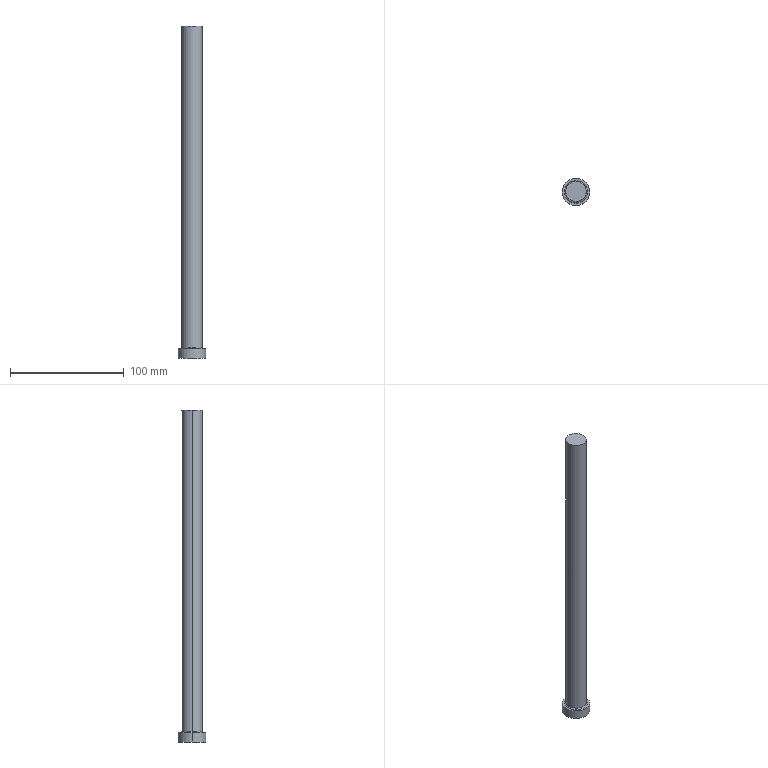Part | STEP file | Pino extrator A - A_18x315 | 1 solid | 9 faces | box 24 x 24 x 292 mm | volume 75901 mm3 | cylinder 4 | plane 3 | torus 2 | commonest cylinder face diameters 18 x2 24 x2
STEP:
#1=CARTESIAN_POINT('',(0.,0.,0.));
#2=DIRECTION('',(0.,0.,1.));
#3=DIRECTION('',(1.,0.,0.));
#4=AXIS2_PLACEMENT_3D('',#1,#2,#3);
#5=CARTESIAN_POINT('',(9.,0.,9.));
#6=VERTEX_POINT('',#5);
#7=CARTESIAN_POINT('',(10.,0.,8.));
#8=VERTEX_POINT('',#7);
#9=CARTESIAN_POINT('',(10.,0.,9.));
#10=DIRECTION('',(0.,-1.,0.));
#11=DIRECTION('',(0.,0.,-1.));
#12=AXIS2_PLACEMENT_3D('',#9,#10,#11);
#13=CIRCLE('',#12,1.);
#14=CARTESIAN_POINT('',(0.,0.,9.));
#15=DIRECTION('',(0.,0.,1.));
#16=DIRECTION('',(1.,0.,0.));
#17=AXIS2_PLACEMENT_3D('',#14,#15,#16);
#18=TOROIDAL_SURFACE('',#17,10.,1.);
#19=CARTESIAN_POINT('',(6.283,-1.571));
#20=DIRECTION('',(0.,1.));
#21=VECTOR('',#20,1.);
#22=LINE('',#19,#21);
#23=(GEOMETRIC_REPRESENTATION_CONTEXT(2)PARAMETRIC_REPRESENTATION_CONTEXT()REPRESENTATION_CONTEXT('',''));
#24=DEFINITIONAL_REPRESENTATION('',(#22),#23);
#25=PCURVE('',#18,#24);
#26=CARTESIAN_POINT('',(0.,0.,9.));
#27=DIRECTION('',(0.,0.,1.));
#28=DIRECTION('',(1.,0.,0.));
#29=AXIS2_PLACEMENT_3D('',#26,#27,#28);
#30=TOROIDAL_SURFACE('',#29,10.,1.);
#31=CARTESIAN_POINT('',(0.,-1.571));
#32=DIRECTION('',(0.,1.));
#33=VECTOR('',#32,1.);
#34=LINE('',#31,#33);
#35=(GEOMETRIC_REPRESENTATION_CONTEXT(2)PARAMETRIC_REPRESENTATION_CONTEXT()REPRESENTATION_CONTEXT('',''));
#36=DEFINITIONAL_REPRESENTATION('',(#34),#35);
#37=PCURVE('',#30,#36);
#38=SURFACE_CURVE('',#13,(#25,#37),.PCURVE_S1.);
#39=EDGE_CURVE('',#6,#8,#38,.T.);
#40=ORIENTED_EDGE('',*,*,#39,.T.);
#41=CARTESIAN_POINT('',(-10.,0.,8.));
#42=VERTEX_POINT('',#41);
#43=CARTESIAN_POINT('',(0.,0.,8.));
#44=DIRECTION('',(0.,0.,-1.));
#45=DIRECTION('',(1.,0.,0.));
#46=AXIS2_PLACEMENT_3D('',#43,#44,#45);
#47=CIRCLE('',#46,10.);
#48=CARTESIAN_POINT('',(6.283,4.712));
#49=DIRECTION('',(-1.,0.));
#50=VECTOR('',#49,1.);
#51=LINE('',#48,#50);
#52=(GEOMETRIC_REPRESENTATION_CONTEXT(2)PARAMETRIC_REPRESENTATION_CONTEXT()REPRESENTATION_CONTEXT('',''));
#53=DEFINITIONAL_REPRESENTATION('',(#51),#52);
#54=PCURVE('',#18,#53);
#55=CARTESIAN_POINT('',(12.,0.,8.));
#56=DIRECTION('',(0.,0.,1.));
#57=DIRECTION('',(1.,0.,0.));
#58=AXIS2_PLACEMENT_3D('',#55,#56,#57);
#59=PLANE('',#58);
#60=CARTESIAN_POINT('',(-2.,0.));
#61=CARTESIAN_POINT('',(-2.,-17.321));
#62=CARTESIAN_POINT('',(-17.,-8.66));
#63=CARTESIAN_POINT('',(-32.,0.));
#64=CARTESIAN_POINT('',(-17.,8.66));
#65=CARTESIAN_POINT('',(-2.,17.321));
#66=CARTESIAN_POINT('',(-2.,0.));
#67=(BOUNDED_CURVE()B_SPLINE_CURVE(2,(#60,#61,#62,#63,#64,#65,#66),.UNSPECIFIED.,.T.,.F.)B_SPLINE_CURVE_WITH_KNOTS((1,2,2,2,2,1),(-2.094,0.,2.094,4.189,6.283,8.378),.UNSPECIFIED.)CURVE()GEOMETRIC_REPRESENTATION_ITEM()RATIONAL_B_SPLINE_CURVE((1.,0.5,1.,0.5,1.,0.5,1.))REPRESENTATION_ITEM(''));
#68=(GEOMETRIC_REPRESENTATION_CONTEXT(2)PARAMETRIC_REPRESENTATION_CONTEXT()REPRESENTATION_CONTEXT('',''));
#69=DEFINITIONAL_REPRESENTATION('',(#67),#68);
#70=PCURVE('',#59,#69);
#71=SURFACE_CURVE('',#47,(#54,#70),.PCURVE_S1.);
#72=EDGE_CURVE('',#8,#42,#71,.T.);
#73=ORIENTED_EDGE('',*,*,#72,.T.);
#74=CARTESIAN_POINT('',(-9.,0.,9.));
#75=VERTEX_POINT('',#74);
#76=CARTESIAN_POINT('',(-10.,0.,9.));
#77=DIRECTION('',(0.,1.,0.));
#78=DIRECTION('',(-1.,0.,0.));
#79=AXIS2_PLACEMENT_3D('',#76,#77,#78);
#80=CIRCLE('',#79,1.);
#81=CARTESIAN_POINT('',(3.142,0.));
#82=DIRECTION('',(0.,1.));
#83=VECTOR('',#82,1.);
#84=LINE('',#81,#83);
#85=(GEOMETRIC_REPRESENTATION_CONTEXT(2)PARAMETRIC_REPRESENTATION_CONTEXT()REPRESENTATION_CONTEXT('',''));
#86=DEFINITIONAL_REPRESENTATION('',(#84),#85);
#87=PCURVE('',#18,#86);
#88=CARTESIAN_POINT('',(3.142,0.));
#89=DIRECTION('',(0.,1.));
#90=VECTOR('',#89,1.);
#91=LINE('',#88,#90);
#92=(GEOMETRIC_REPRESENTATION_CONTEXT(2)PARAMETRIC_REPRESENTATION_CONTEXT()REPRESENTATION_CONTEXT('',''));
#93=DEFINITIONAL_REPRESENTATION('',(#91),#92);
#94=PCURVE('',#30,#93);
#95=SURFACE_CURVE('',#80,(#87,#94),.PCURVE_S1.);
#96=EDGE_CURVE('',#75,#42,#95,.T.);
#97=ORIENTED_EDGE('',*,*,#96,.F.);
#98=CARTESIAN_POINT('',(0.,0.,9.));
#99=DIRECTION('',(0.,0.,1.));
#100=DIRECTION('',(1.,0.,0.));
#101=AXIS2_PLACEMENT_3D('',#98,#99,#100);
#102=CIRCLE('',#101,9.);
#103=CARTESIAN_POINT('',(0.,3.142));
#104=DIRECTION('',(1.,0.));
#105=VECTOR('',#104,1.);
#106=LINE('',#103,#105);
#107=(GEOMETRIC_REPRESENTATION_CONTEXT(2)PARAMETRIC_REPRESENTATION_CONTEXT()REPRESENTATION_CONTEXT('',''));
#108=DEFINITIONAL_REPRESENTATION('',(#106),#107);
#109=PCURVE('',#18,#108);
#110=CARTESIAN_POINT('',(0.,0.,0.));
#111=DIRECTION('',(0.,0.,-1.));
#112=DIRECTION('',(-1.,0.,0.));
#113=AXIS2_PLACEMENT_3D('',#110,#111,#112);
#114=CYLINDRICAL_SURFACE('',#113,9.);
#115=CARTESIAN_POINT('',(9.425,-9.));
#116=DIRECTION('',(-1.,0.));
#117=VECTOR('',#116,1.);
#118=LINE('',#115,#117);
#119=(GEOMETRIC_REPRESENTATION_CONTEXT(2)PARAMETRIC_REPRESENTATION_CONTEXT()REPRESENTATION_CONTEXT('',''));
#120=DEFINITIONAL_REPRESENTATION('',(#118),#119);
#121=PCURVE('',#114,#120);
#122=SURFACE_CURVE('',#102,(#109,#121),.PCURVE_S1.);
#123=EDGE_CURVE('',#75,#6,#122,.T.);
#124=ORIENTED_EDGE('',*,*,#123,.T.);
#125=EDGE_LOOP('',(#40,#73,#97,#124));
#126=FACE_BOUND('',#125,.F.);
#127=ADVANCED_FACE('',(#126),#18,.F.);
#128=CARTESIAN_POINT('',(-12.,0.,8.));
#129=VERTEX_POINT('',#128);
#130=CARTESIAN_POINT('',(12.,0.,8.));
#131=VERTEX_POINT('',#130);
#132=CARTESIAN_POINT('',(0.,0.,8.));
#133=DIRECTION('',(0.,0.,-1.));
#134=DIRECTION('',(-1.,0.,0.));
#135=AXIS2_PLACEMENT_3D('',#132,#133,#134);
#136=CIRCLE('',#135,12.);
#137=CARTESIAN_POINT('',(0.,0.,0.));
#138=DIRECTION('',(0.,0.,-1.));
#139=DIRECTION('',(-1.,0.,0.));
#140=AXIS2_PLACEMENT_3D('',#137,#138,#139);
#141=CYLINDRICAL_SURFACE('',#140,12.);
#142=CARTESIAN_POINT('',(0.,-8.));
#143=DIRECTION('',(1.,0.));
#144=VECTOR('',#143,1.);
#145=LINE('',#142,#144);
#146=(GEOMETRIC_REPRESENTATION_CONTEXT(2)PARAMETRIC_REPRESENTATION_CONTEXT()REPRESENTATION_CONTEXT('',''));
#147=DEFINITIONAL_REPRESENTATION('',(#145),#146);
#148=PCURVE('',#141,#147);
#149=CARTESIAN_POINT('',(-24.,0.));
#150=CARTESIAN_POINT('',(-24.,20.785));
#151=CARTESIAN_POINT('',(-6.,10.392));
#152=CARTESIAN_POINT('',(12.,0.));
#153=CARTESIAN_POINT('',(-6.,-10.392));
#154=CARTESIAN_POINT('',(-24.,-20.785));
#155=CARTESIAN_POINT('',(-24.,0.));
#156=(BOUNDED_CURVE()B_SPLINE_CURVE(2,(#149,#150,#151,#152,#153,#154,#155),.UNSPECIFIED.,.T.,.F.)B_SPLINE_CURVE_WITH_KNOTS((1,2,2,2,2,1),(-2.094,0.,2.094,4.189,6.283,8.378),.UNSPECIFIED.)CURVE()GEOMETRIC_REPRESENTATION_ITEM()RATIONAL_B_SPLINE_CURVE((1.,0.5,1.,0.5,1.,0.5,1.))REPRESENTATION_ITEM(''));
#157=(GEOMETRIC_REPRESENTATION_CONTEXT(2)PARAMETRIC_REPRESENTATION_CONTEXT()REPRESENTATION_CONTEXT('',''));
#158=DEFINITIONAL_REPRESENTATION('',(#156),#157);
#159=PCURVE('',#59,#158);
#160=SURFACE_CURVE('',#136,(#148,#159),.PCURVE_S1.);
#161=EDGE_CURVE('',#129,#131,#160,.T.);
#162=ORIENTED_EDGE('',*,*,#161,.T.);
#163=CARTESIAN_POINT('',(12.,0.,0.));
#164=VERTEX_POINT('',#163);
#165=CARTESIAN_POINT('',(12.,0.,0.));
#166=DIRECTION('',(0.,0.,-1.));
#167=VECTOR('',#166,1.);
#168=LINE('',#165,#167);
#169=CARTESIAN_POINT('',(3.142,0.));
#170=DIRECTION('',(0.,1.));
#171=VECTOR('',#170,1.);
#172=LINE('',#169,#171);
#173=(GEOMETRIC_REPRESENTATION_CONTEXT(2)PARAMETRIC_REPRESENTATION_CONTEXT()REPRESENTATION_CONTEXT('',''));
#174=DEFINITIONAL_REPRESENTATION('',(#172),#173);
#175=PCURVE('',#141,#174);
#176=CARTESIAN_POINT('',(0.,0.,0.));
#177=DIRECTION('',(0.,0.,-1.));
#178=DIRECTION('',(-1.,0.,0.));
#179=AXIS2_PLACEMENT_3D('',#176,#177,#178);
#180=CYLINDRICAL_SURFACE('',#179,12.);
#181=CARTESIAN_POINT('',(3.142,0.));
#182=DIRECTION('',(0.,1.));
#183=VECTOR('',#182,1.);
#184=LINE('',#181,#183);
#185=(GEOMETRIC_REPRESENTATION_CONTEXT(2)PARAMETRIC_REPRESENTATION_CONTEXT()REPRESENTATION_CONTEXT('',''));
#186=DEFINITIONAL_REPRESENTATION('',(#184),#185);
#187=PCURVE('',#180,#186);
#188=SURFACE_CURVE('',#168,(#175,#187),.PCURVE_S1.);
#189=EDGE_CURVE('',#131,#164,#188,.T.);
#190=ORIENTED_EDGE('',*,*,#189,.T.);
#191=CARTESIAN_POINT('',(-12.,0.,0.));
#192=VERTEX_POINT('',#191);
#193=CARTESIAN_POINT('',(0.,0.,0.));
#194=DIRECTION('',(0.,0.,-1.));
#195=DIRECTION('',(-1.,0.,0.));
#196=AXIS2_PLACEMENT_3D('',#193,#194,#195);
#197=CIRCLE('',#196,12.);
#198=CARTESIAN_POINT('',(0.,0.));
#199=DIRECTION('',(1.,0.));
#200=VECTOR('',#199,1.);
#201=LINE('',#198,#200);
#202=(GEOMETRIC_REPRESENTATION_CONTEXT(2)PARAMETRIC_REPRESENTATION_CONTEXT()REPRESENTATION_CONTEXT('',''));
#203=DEFINITIONAL_REPRESENTATION('',(#201),#202);
#204=PCURVE('',#141,#203);
#205=CARTESIAN_POINT('',(0.,0.,0.));
#206=DIRECTION('',(0.,0.,-1.));
#207=DIRECTION('',(-1.,0.,0.));
#208=AXIS2_PLACEMENT_3D('',#205,#206,#207);
#209=PLANE('',#208);
#210=CARTESIAN_POINT('',(0.,0.));
#211=DIRECTION('',(1.,0.));
#212=AXIS2_PLACEMENT_2D('',#210,#211);
#213=CIRCLE('',#212,12.);
#214=(GEOMETRIC_REPRESENTATION_CONTEXT(2)PARAMETRIC_REPRESENTATION_CONTEXT()REPRESENTATION_CONTEXT('',''));
#215=DEFINITIONAL_REPRESENTATION('',(#213),#214);
#216=PCURVE('',#209,#215);
#217=SURFACE_CURVE('',#197,(#204,#216),.PCURVE_S1.);
#218=EDGE_CURVE('',#192,#164,#217,.T.);
#219=ORIENTED_EDGE('',*,*,#218,.F.);
#220=CARTESIAN_POINT('',(-12.,0.,0.));
#221=DIRECTION('',(0.,0.,-1.));
#222=VECTOR('',#221,1.);
#223=LINE('',#220,#222);
#224=CARTESIAN_POINT('',(0.,0.));
#225=DIRECTION('',(0.,1.));
#226=VECTOR('',#225,1.);
#227=LINE('',#224,#226);
#228=(GEOMETRIC_REPRESENTATION_CONTEXT(2)PARAMETRIC_REPRESENTATION_CONTEXT()REPRESENTATION_CONTEXT('',''));
#229=DEFINITIONAL_REPRESENTATION('',(#227),#228);
#230=PCURVE('',#141,#229);
#231=CARTESIAN_POINT('',(6.283,0.));
#232=DIRECTION('',(0.,1.));
#233=VECTOR('',#232,1.);
#234=LINE('',#231,#233);
#235=(GEOMETRIC_REPRESENTATION_CONTEXT(2)PARAMETRIC_REPRESENTATION_CONTEXT()REPRESENTATION_CONTEXT('',''));
#236=DEFINITIONAL_REPRESENTATION('',(#234),#235);
#237=PCURVE('',#180,#236);
#238=SURFACE_CURVE('',#223,(#230,#237),.PCURVE_S1.);
#239=EDGE_CURVE('',#129,#192,#238,.T.);
#240=ORIENTED_EDGE('',*,*,#239,.F.);
#241=EDGE_LOOP('',(#162,#190,#219,#240));
#242=FACE_BOUND('',#241,.T.);
#243=ADVANCED_FACE('',(#242),#141,.T.);
#244=CARTESIAN_POINT('',(9.,0.,292.));
#245=VERTEX_POINT('',#244);
#246=CARTESIAN_POINT('',(-9.,0.,292.));
#247=VERTEX_POINT('',#246);
#248=CARTESIAN_POINT('',(0.,0.,292.));
#249=DIRECTION('',(0.,0.,1.));
#250=DIRECTION('',(1.,0.,0.));
#251=AXIS2_PLACEMENT_3D('',#248,#249,#250);
#252=CIRCLE('',#251,9.);
#253=CARTESIAN_POINT('',(0.,0.,0.));
#254=DIRECTION('',(0.,0.,-1.));
#255=DIRECTION('',(-1.,0.,0.));
#256=AXIS2_PLACEMENT_3D('',#253,#254,#255);
#257=CYLINDRICAL_SURFACE('',#256,9.);
#258=CARTESIAN_POINT('',(3.142,-292.));
#259=DIRECTION('',(-1.,0.));
#260=VECTOR('',#259,1.);
#261=LINE('',#258,#260);
#262=(GEOMETRIC_REPRESENTATION_CONTEXT(2)PARAMETRIC_REPRESENTATION_CONTEXT()REPRESENTATION_CONTEXT('',''));
#263=DEFINITIONAL_REPRESENTATION('',(#261),#262);
#264=PCURVE('',#257,#263);
#265=CARTESIAN_POINT('',(0.,0.,292.));
#266=DIRECTION('',(0.,0.,1.));
#267=DIRECTION('',(1.,0.,0.));
#268=AXIS2_PLACEMENT_3D('',#265,#266,#267);
#269=PLANE('',#268);
#270=CARTESIAN_POINT('',(0.,0.));
#271=DIRECTION('',(1.,0.));
#272=AXIS2_PLACEMENT_2D('',#270,#271);
#273=CIRCLE('',#272,9.);
#274=(GEOMETRIC_REPRESENTATION_CONTEXT(2)PARAMETRIC_REPRESENTATION_CONTEXT()REPRESENTATION_CONTEXT('',''));
#275=DEFINITIONAL_REPRESENTATION('',(#273),#274);
#276=PCURVE('',#269,#275);
#277=SURFACE_CURVE('',#252,(#264,#276),.PCURVE_S1.);
#278=EDGE_CURVE('',#245,#247,#277,.T.);
#279=ORIENTED_EDGE('',*,*,#278,.F.);
#280=CARTESIAN_POINT('',(9.,0.,0.));
#281=DIRECTION('',(0.,0.,-1.));
#282=VECTOR('',#281,1.);
#283=LINE('',#280,#282);
#284=CARTESIAN_POINT('',(3.142,0.));
#285=DIRECTION('',(0.,1.));
#286=VECTOR('',#285,1.);
#287=LINE('',#284,#286);
#288=(GEOMETRIC_REPRESENTATION_CONTEXT(2)PARAMETRIC_REPRESENTATION_CONTEXT()REPRESENTATION_CONTEXT('',''));
#289=DEFINITIONAL_REPRESENTATION('',(#287),#288);
#290=PCURVE('',#257,#289);
#291=CARTESIAN_POINT('',(3.142,0.));
#292=DIRECTION('',(0.,1.));
#293=VECTOR('',#292,1.);
#294=LINE('',#291,#293);
#295=(GEOMETRIC_REPRESENTATION_CONTEXT(2)PARAMETRIC_REPRESENTATION_CONTEXT()REPRESENTATION_CONTEXT('',''));
#296=DEFINITIONAL_REPRESENTATION('',(#294),#295);
#297=PCURVE('',#114,#296);
#298=SURFACE_CURVE('',#283,(#290,#297),.PCURVE_S1.);
#299=EDGE_CURVE('',#245,#6,#298,.T.);
#300=ORIENTED_EDGE('',*,*,#299,.T.);
#301=CARTESIAN_POINT('',(0.,0.,9.));
#302=DIRECTION('',(0.,0.,1.));
#303=DIRECTION('',(1.,0.,0.));
#304=AXIS2_PLACEMENT_3D('',#301,#302,#303);
#305=CIRCLE('',#304,9.);
#306=CARTESIAN_POINT('',(3.142,-9.));
#307=DIRECTION('',(-1.,0.));
#308=VECTOR('',#307,1.);
#309=LINE('',#306,#308);
#310=(GEOMETRIC_REPRESENTATION_CONTEXT(2)PARAMETRIC_REPRESENTATION_CONTEXT()REPRESENTATION_CONTEXT('',''));
#311=DEFINITIONAL_REPRESENTATION('',(#309),#310);
#312=PCURVE('',#257,#311);
#313=CARTESIAN_POINT('',(0.,3.142));
#314=DIRECTION('',(1.,0.));
#315=VECTOR('',#314,1.);
#316=LINE('',#313,#315);
#317=(GEOMETRIC_REPRESENTATION_CONTEXT(2)PARAMETRIC_REPRESENTATION_CONTEXT()REPRESENTATION_CONTEXT('',''));
#318=DEFINITIONAL_REPRESENTATION('',(#316),#317);
#319=PCURVE('',#30,#318);
#320=SURFACE_CURVE('',#305,(#312,#319),.PCURVE_S1.);
#321=EDGE_CURVE('',#6,#75,#320,.T.);
#322=ORIENTED_EDGE('',*,*,#321,.T.);
#323=CARTESIAN_POINT('',(-9.,0.,0.));
#324=DIRECTION('',(0.,0.,-1.));
#325=VECTOR('',#324,1.);
#326=LINE('',#323,#325);
#327=CARTESIAN_POINT('',(0.,0.));
#328=DIRECTION('',(0.,1.));
#329=VECTOR('',#328,1.);
#330=LINE('',#327,#329);
#331=(GEOMETRIC_REPRESENTATION_CONTEXT(2)PARAMETRIC_REPRESENTATION_CONTEXT()REPRESENTATION_CONTEXT('',''));
#332=DEFINITIONAL_REPRESENTATION('',(#330),#331);
#333=PCURVE('',#257,#332);
#334=CARTESIAN_POINT('',(6.283,0.));
#335=DIRECTION('',(0.,1.));
#336=VECTOR('',#335,1.);
#337=LINE('',#334,#336);
#338=(GEOMETRIC_REPRESENTATION_CONTEXT(2)PARAMETRIC_REPRESENTATION_CONTEXT()REPRESENTATION_CONTEXT('',''));
#339=DEFINITIONAL_REPRESENTATION('',(#337),#338);
#340=PCURVE('',#114,#339);
#341=SURFACE_CURVE('',#326,(#333,#340),.PCURVE_S1.);
#342=EDGE_CURVE('',#247,#75,#341,.T.);
#343=ORIENTED_EDGE('',*,*,#342,.F.);
#344=EDGE_LOOP('',(#279,#300,#322,#343));
#345=FACE_BOUND('',#344,.T.);
#346=ADVANCED_FACE('',(#345),#257,.T.);
#347=ORIENTED_EDGE('',*,*,#299,.F.);
#348=CARTESIAN_POINT('',(0.,0.,292.));
#349=DIRECTION('',(0.,0.,1.));
#350=DIRECTION('',(1.,0.,0.));
#351=AXIS2_PLACEMENT_3D('',#348,#349,#350);
#352=CIRCLE('',#351,9.);
#353=CARTESIAN_POINT('',(9.425,-292.));
#354=DIRECTION('',(-1.,0.));
#355=VECTOR('',#354,1.);
#356=LINE('',#353,#355);
#357=(GEOMETRIC_REPRESENTATION_CONTEXT(2)PARAMETRIC_REPRESENTATION_CONTEXT()REPRESENTATION_CONTEXT('',''));
#358=DEFINITIONAL_REPRESENTATION('',(#356),#357);
#359=PCURVE('',#114,#358);
#360=CARTESIAN_POINT('',(0.,0.));
#361=DIRECTION('',(1.,0.));
#362=AXIS2_PLACEMENT_2D('',#360,#361);
#363=CIRCLE('',#362,9.);
#364=(GEOMETRIC_REPRESENTATION_CONTEXT(2)PARAMETRIC_REPRESENTATION_CONTEXT()REPRESENTATION_CONTEXT('',''));
#365=DEFINITIONAL_REPRESENTATION('',(#363),#364);
#366=PCURVE('',#269,#365);
#367=SURFACE_CURVE('',#352,(#359,#366),.PCURVE_S1.);
#368=EDGE_CURVE('',#247,#245,#367,.T.);
#369=ORIENTED_EDGE('',*,*,#368,.F.);
#370=ORIENTED_EDGE('',*,*,#342,.T.);
#371=ORIENTED_EDGE('',*,*,#123,.T.);
#372=EDGE_LOOP('',(#347,#369,#370,#371));
#373=FACE_BOUND('',#372,.T.);
#374=ADVANCED_FACE('',(#373),#114,.T.);
#375=ORIENTED_EDGE('',*,*,#218,.T.);
#376=CARTESIAN_POINT('',(0.,0.,0.));
#377=DIRECTION('',(0.,0.,-1.));
#378=DIRECTION('',(-1.,0.,0.));
#379=AXIS2_PLACEMENT_3D('',#376,#377,#378);
#380=CIRCLE('',#379,12.);
#381=CARTESIAN_POINT('',(0.,0.));
#382=DIRECTION('',(1.,0.));
#383=AXIS2_PLACEMENT_2D('',#381,#382);
#384=CIRCLE('',#383,12.);
#385=(GEOMETRIC_REPRESENTATION_CONTEXT(2)PARAMETRIC_REPRESENTATION_CONTEXT()REPRESENTATION_CONTEXT('',''));
#386=DEFINITIONAL_REPRESENTATION('',(#384),#385);
#387=PCURVE('',#209,#386);
#388=CARTESIAN_POINT('',(0.,0.));
#389=DIRECTION('',(1.,0.));
#390=VECTOR('',#389,1.);
#391=LINE('',#388,#390);
#392=(GEOMETRIC_REPRESENTATION_CONTEXT(2)PARAMETRIC_REPRESENTATION_CONTEXT()REPRESENTATION_CONTEXT('',''));
#393=DEFINITIONAL_REPRESENTATION('',(#391),#392);
#394=PCURVE('',#180,#393);
#395=SURFACE_CURVE('',#380,(#387,#394),.PCURVE_S1.);
#396=EDGE_CURVE('',#164,#192,#395,.T.);
#397=ORIENTED_EDGE('',*,*,#396,.T.);
#398=EDGE_LOOP('',(#375,#397));
#399=FACE_BOUND('',#398,.T.);
#400=ADVANCED_FACE('',(#399),#209,.T.);
#401=ORIENTED_EDGE('',*,*,#189,.F.);
#402=CARTESIAN_POINT('',(0.,0.,8.));
#403=DIRECTION('',(0.,0.,-1.));
#404=DIRECTION('',(-1.,0.,0.));
#405=AXIS2_PLACEMENT_3D('',#402,#403,#404);
#406=CIRCLE('',#405,12.);
#407=CARTESIAN_POINT('',(0.,-8.));
#408=DIRECTION('',(1.,0.));
#409=VECTOR('',#408,1.);
#410=LINE('',#407,#409);
#411=(GEOMETRIC_REPRESENTATION_CONTEXT(2)PARAMETRIC_REPRESENTATION_CONTEXT()REPRESENTATION_CONTEXT('',''));
#412=DEFINITIONAL_REPRESENTATION('',(#410),#411);
#413=PCURVE('',#180,#412);
#414=CARTESIAN_POINT('',(-24.,0.));
#415=CARTESIAN_POINT('',(-24.,20.785));
#416=CARTESIAN_POINT('',(-6.,10.392));
#417=CARTESIAN_POINT('',(12.,0.));
#418=CARTESIAN_POINT('',(-6.,-10.392));
#419=CARTESIAN_POINT('',(-24.,-20.785));
#420=CARTESIAN_POINT('',(-24.,0.));
#421=(BOUNDED_CURVE()B_SPLINE_CURVE(2,(#414,#415,#416,#417,#418,#419,#420),.UNSPECIFIED.,.T.,.F.)B_SPLINE_CURVE_WITH_KNOTS((1,2,2,2,2,1),(-2.094,0.,2.094,4.189,6.283,8.378),.UNSPECIFIED.)CURVE()GEOMETRIC_REPRESENTATION_ITEM()RATIONAL_B_SPLINE_CURVE((1.,0.5,1.,0.5,1.,0.5,1.))REPRESENTATION_ITEM(''));
#422=(GEOMETRIC_REPRESENTATION_CONTEXT(2)PARAMETRIC_REPRESENTATION_CONTEXT()REPRESENTATION_CONTEXT('',''));
#423=DEFINITIONAL_REPRESENTATION('',(#421),#422);
#424=PCURVE('',#59,#423);
#425=SURFACE_CURVE('',#406,(#413,#424),.PCURVE_S1.);
#426=EDGE_CURVE('',#131,#129,#425,.T.);
#427=ORIENTED_EDGE('',*,*,#426,.T.);
#428=ORIENTED_EDGE('',*,*,#239,.T.);
#429=ORIENTED_EDGE('',*,*,#396,.F.);
#430=EDGE_LOOP('',(#401,#427,#428,#429));
#431=FACE_BOUND('',#430,.T.);
#432=ADVANCED_FACE('',(#431),#180,.T.);
#433=ORIENTED_EDGE('',*,*,#72,.T.);
#434=CARTESIAN_POINT('',(0.,0.,8.));
#435=DIRECTION('',(0.,0.,-1.));
#436=DIRECTION('',(1.,0.,0.));
#437=AXIS2_PLACEMENT_3D('',#434,#435,#436);
#438=CIRCLE('',#437,10.);
#439=CARTESIAN_POINT('',(-2.,0.));
#440=CARTESIAN_POINT('',(-2.,-17.321));
#441=CARTESIAN_POINT('',(-17.,-8.66));
#442=CARTESIAN_POINT('',(-32.,0.));
#443=CARTESIAN_POINT('',(-17.,8.66));
#444=CARTESIAN_POINT('',(-2.,17.321));
#445=CARTESIAN_POINT('',(-2.,0.));
#446=(BOUNDED_CURVE()B_SPLINE_CURVE(2,(#439,#440,#441,#442,#443,#444,#445),.UNSPECIFIED.,.T.,.F.)B_SPLINE_CURVE_WITH_KNOTS((1,2,2,2,2,1),(-2.094,0.,2.094,4.189,6.283,8.378),.UNSPECIFIED.)CURVE()GEOMETRIC_REPRESENTATION_ITEM()RATIONAL_B_SPLINE_CURVE((1.,0.5,1.,0.5,1.,0.5,1.))REPRESENTATION_ITEM(''));
#447=(GEOMETRIC_REPRESENTATION_CONTEXT(2)PARAMETRIC_REPRESENTATION_CONTEXT()REPRESENTATION_CONTEXT('',''));
#448=DEFINITIONAL_REPRESENTATION('',(#446),#447);
#449=PCURVE('',#59,#448);
#450=CARTESIAN_POINT('',(6.283,4.712));
#451=DIRECTION('',(-1.,0.));
#452=VECTOR('',#451,1.);
#453=LINE('',#450,#452);
#454=(GEOMETRIC_REPRESENTATION_CONTEXT(2)PARAMETRIC_REPRESENTATION_CONTEXT()REPRESENTATION_CONTEXT('',''));
#455=DEFINITIONAL_REPRESENTATION('',(#453),#454);
#456=PCURVE('',#30,#455);
#457=SURFACE_CURVE('',#438,(#449,#456),.PCURVE_S1.);
#458=EDGE_CURVE('',#42,#8,#457,.T.);
#459=ORIENTED_EDGE('',*,*,#458,.T.);
#460=EDGE_LOOP('',(#433,#459));
#461=FACE_BOUND('',#460,.T.);
#462=ORIENTED_EDGE('',*,*,#161,.F.);
#463=ORIENTED_EDGE('',*,*,#426,.F.);
#464=EDGE_LOOP('',(#462,#463));
#465=FACE_BOUND('',#464,.T.);
#466=ADVANCED_FACE('',(#461,#465),#59,.T.);
#467=ORIENTED_EDGE('',*,*,#458,.T.);
#468=ORIENTED_EDGE('',*,*,#39,.F.);
#469=ORIENTED_EDGE('',*,*,#321,.T.);
#470=ORIENTED_EDGE('',*,*,#96,.T.);
#471=EDGE_LOOP('',(#467,#468,#469,#470));
#472=FACE_BOUND('',#471,.F.);
#473=ADVANCED_FACE('',(#472),#30,.F.);
#474=ORIENTED_EDGE('',*,*,#368,.T.);
#475=ORIENTED_EDGE('',*,*,#278,.T.);
#476=EDGE_LOOP('',(#474,#475));
#477=FACE_BOUND('',#476,.T.);
#478=ADVANCED_FACE('',(#477),#269,.T.);
#479=CLOSED_SHELL('',(#127,#243,#346,#374,#400,#432,#466,#473,#478));
#480=MANIFOLD_SOLID_BREP('',#479);
#481=(LENGTH_UNIT()NAMED_UNIT(*)SI_UNIT(.MILLI.,.METRE.));
#482=UNCERTAINTY_MEASURE_WITH_UNIT(LENGTH_MEASURE(0.0000001),#481,'','');
#483=(NAMED_UNIT(*)PLANE_ANGLE_UNIT()SI_UNIT($,.RADIAN.));
#484=(NAMED_UNIT(*)SI_UNIT($,.STERADIAN.)SOLID_ANGLE_UNIT());
#485=(GEOMETRIC_REPRESENTATION_CONTEXT(3)GLOBAL_UNCERTAINTY_ASSIGNED_CONTEXT((#482))GLOBAL_UNIT_ASSIGNED_CONTEXT((#481,#483,#484))REPRESENTATION_CONTEXT('',''));
#486=ADVANCED_BREP_SHAPE_REPRESENTATION('',(#4,#480),#485);